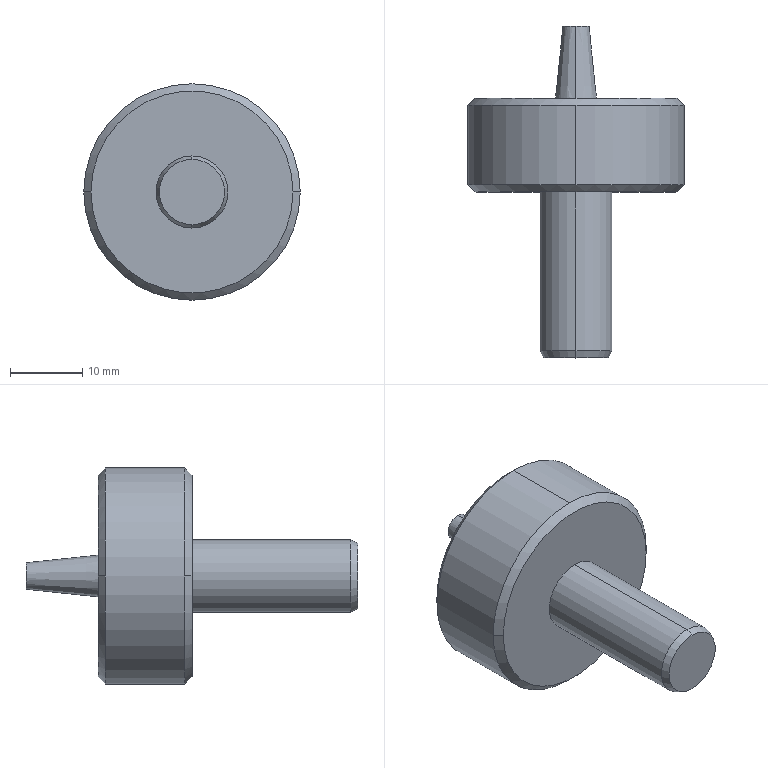Part | SolidWorks | features BaseBody 1 | 1 solid | 19 faces | box 30 x 46 x 30 mm | volume 10612 mm3 | cone 8 | cylinder 6 | plane 5 | commonest cylinder face diameters 10 x2 25 x2 30 x2
STEP:
#1=CARTESIAN_POINT('',(-418.,-55.,252.121));
#2=VERTEX_POINT('',#1);
#3=CARTESIAN_POINT('',(-418.,-55.,242.121));
#4=VERTEX_POINT('',#3);
#5=CARTESIAN_POINT('',(-418.,-55.,247.121));
#6=DIRECTION('',(0.,1.,0.));
#7=DIRECTION('',(0.,0.,-1.));
#8=AXIS2_PLACEMENT_3D('',#5,#6,#7);
#9=CIRCLE('',#8,5.);
#10=EDGE_CURVE('',#2,#4,#9,.T.);
#11=ORIENTED_EDGE('',*,*,#10,.F.);
#12=CARTESIAN_POINT('',(-418.,-77.,252.121));
#13=VERTEX_POINT('',#12);
#14=CARTESIAN_POINT('',(-418.,-78.,252.121));
#15=DIRECTION('',(0.,-1.,0.));
#16=VECTOR('',#15,1000.);
#17=LINE('',#14,#16);
#18=EDGE_CURVE('',#2,#13,#17,.T.);
#19=ORIENTED_EDGE('',*,*,#18,.T.);
#20=CARTESIAN_POINT('',(-418.,-77.,242.121));
#21=VERTEX_POINT('',#20);
#22=CARTESIAN_POINT('',(-418.,-77.,247.121));
#23=DIRECTION('',(0.,1.,0.));
#24=DIRECTION('',(0.,0.,-1.));
#25=AXIS2_PLACEMENT_3D('',#22,#23,#24);
#26=CIRCLE('',#25,5.);
#27=EDGE_CURVE('',#13,#21,#26,.T.);
#28=ORIENTED_EDGE('',*,*,#27,.T.);
#29=CARTESIAN_POINT('',(-418.,-78.,242.121));
#30=DIRECTION('',(0.,-1.,0.));
#31=VECTOR('',#30,1000.);
#32=LINE('',#29,#31);
#33=EDGE_CURVE('',#4,#21,#32,.T.);
#34=ORIENTED_EDGE('',*,*,#33,.F.);
#35=EDGE_LOOP('',(#11,#19,#28,#34));
#36=FACE_OUTER_BOUND('',#35,.T.);
#37=CARTESIAN_POINT('',(-418.,-78.,247.121));
#38=DIRECTION('',(0.,-1.,0.));
#39=DIRECTION('',(0.,0.,-1.));
#40=AXIS2_PLACEMENT_3D('',#37,#38,#39);
#41=CYLINDRICAL_SURFACE('',#40,5.);
#42=ADVANCED_FACE('',(#36),#41,.T.);
#43=CARTESIAN_POINT('',(-404.,-55.,247.121));
#44=VERTEX_POINT('',#43);
#45=CARTESIAN_POINT('',(-432.,-55.,247.121));
#46=VERTEX_POINT('',#45);
#47=CARTESIAN_POINT('',(-418.,-55.,247.121));
#48=DIRECTION('',(0.,-1.,0.));
#49=DIRECTION('',(-1.,0.,0.));
#50=AXIS2_PLACEMENT_3D('',#47,#48,#49);
#51=CIRCLE('',#50,14.);
#52=EDGE_CURVE('',#44,#46,#51,.T.);
#53=ORIENTED_EDGE('',*,*,#52,.F.);
#54=CARTESIAN_POINT('',(-403.,-54.,247.121));
#55=VERTEX_POINT('',#54);
#56=CARTESIAN_POINT('',(-403.,-54.,247.121));
#57=DIRECTION('',(0.7071,0.7071,0.));
#58=VECTOR('',#57,1000.);
#59=LINE('',#56,#58);
#60=EDGE_CURVE('',#44,#55,#59,.T.);
#61=ORIENTED_EDGE('',*,*,#60,.T.);
#62=CARTESIAN_POINT('',(-418.,-54.,262.121));
#63=VERTEX_POINT('',#62);
#64=CARTESIAN_POINT('',(-418.,-54.,247.121));
#65=DIRECTION('',(0.,-1.,0.));
#66=DIRECTION('',(0.114,0.,-0.9935));
#67=AXIS2_PLACEMENT_3D('',#64,#65,#66);
#68=CIRCLE('',#67,15.);
#69=EDGE_CURVE('',#55,#63,#68,.T.);
#70=ORIENTED_EDGE('',*,*,#69,.T.);
#71=CARTESIAN_POINT('',(-433.,-54.,247.121));
#72=VERTEX_POINT('',#71);
#73=CARTESIAN_POINT('',(-418.,-54.,247.121));
#74=DIRECTION('',(0.,-1.,0.));
#75=DIRECTION('',(0.114,0.,-0.9935));
#76=AXIS2_PLACEMENT_3D('',#73,#74,#75);
#77=CIRCLE('',#76,15.);
#78=EDGE_CURVE('',#63,#72,#77,.T.);
#79=ORIENTED_EDGE('',*,*,#78,.T.);
#80=CARTESIAN_POINT('',(-433.,-54.,247.121));
#81=DIRECTION('',(-0.7071,0.7071,0.));
#82=VECTOR('',#81,1000.);
#83=LINE('',#80,#82);
#84=EDGE_CURVE('',#46,#72,#83,.T.);
#85=ORIENTED_EDGE('',*,*,#84,.F.);
#86=EDGE_LOOP('',(#53,#61,#70,#79,#85));
#87=FACE_OUTER_BOUND('',#86,.T.);
#88=CARTESIAN_POINT('',(-418.,-54.,247.121));
#89=DIRECTION('',(0.,1.,0.));
#90=DIRECTION('',(-1.,0.,0.));
#91=AXIS2_PLACEMENT_3D('',#88,#89,#90);
#92=CONICAL_SURFACE('',#91,15.,0.7854);
#93=ADVANCED_FACE('',(#87),#92,.T.);
#94=CARTESIAN_POINT('',(-418.,-78.,251.655));
#95=VERTEX_POINT('',#94);
#96=CARTESIAN_POINT('',(-418.,-78.,242.587));
#97=VERTEX_POINT('',#96);
#98=CARTESIAN_POINT('',(-418.,-78.,247.121));
#99=DIRECTION('',(0.,1.,0.));
#100=DIRECTION('',(0.,0.,1.));
#101=AXIS2_PLACEMENT_3D('',#98,#99,#100);
#102=CIRCLE('',#101,4.534);
#103=EDGE_CURVE('',#95,#97,#102,.T.);
#104=ORIENTED_EDGE('',*,*,#103,.T.);
#105=CARTESIAN_POINT('',(-418.,-77.,242.121));
#106=DIRECTION('',(0.,0.9063,-0.4226));
#107=VECTOR('',#106,1000.);
#108=LINE('',#105,#107);
#109=EDGE_CURVE('',#97,#21,#108,.T.);
#110=ORIENTED_EDGE('',*,*,#109,.T.);
#111=ORIENTED_EDGE('',*,*,#27,.F.);
#112=CARTESIAN_POINT('',(-418.,-77.,252.121));
#113=DIRECTION('',(0.,0.9063,0.4226));
#114=VECTOR('',#113,1000.);
#115=LINE('',#112,#114);
#116=EDGE_CURVE('',#95,#13,#115,.T.);
#117=ORIENTED_EDGE('',*,*,#116,.F.);
#118=EDGE_LOOP('',(#104,#110,#111,#117));
#119=FACE_OUTER_BOUND('',#118,.T.);
#120=CARTESIAN_POINT('',(-418.,-77.,247.121));
#121=DIRECTION('',(0.,1.,0.));
#122=DIRECTION('',(0.,0.,1.));
#123=AXIS2_PLACEMENT_3D('',#120,#121,#122);
#124=CONICAL_SURFACE('',#123,5.,0.4363);
#125=ADVANCED_FACE('',(#119),#124,.T.);
#126=CARTESIAN_POINT('',(-403.,-43.,247.121));
#127=VERTEX_POINT('',#126);
#128=CARTESIAN_POINT('',(-418.,-43.,262.121));
#129=VERTEX_POINT('',#128);
#130=CARTESIAN_POINT('',(-418.,-43.,247.121));
#131=DIRECTION('',(0.,-1.,0.));
#132=DIRECTION('',(0.,0.,-1.));
#133=AXIS2_PLACEMENT_3D('',#130,#131,#132);
#134=CIRCLE('',#133,15.);
#135=EDGE_CURVE('',#127,#129,#134,.T.);
#136=ORIENTED_EDGE('',*,*,#135,.T.);
#137=CARTESIAN_POINT('',(-418.,-78.,262.121));
#138=DIRECTION('',(0.,-1.,0.));
#139=VECTOR('',#138,1000.);
#140=LINE('',#137,#139);
#141=EDGE_CURVE('',#129,#63,#140,.T.);
#142=ORIENTED_EDGE('',*,*,#141,.T.);
#143=ORIENTED_EDGE('',*,*,#69,.F.);
#144=CARTESIAN_POINT('',(-418.,-54.,232.121));
#145=VERTEX_POINT('',#144);
#146=CARTESIAN_POINT('',(-418.,-54.,247.121));
#147=DIRECTION('',(0.,-1.,0.));
#148=DIRECTION('',(0.114,0.,-0.9935));
#149=AXIS2_PLACEMENT_3D('',#146,#147,#148);
#150=CIRCLE('',#149,15.);
#151=EDGE_CURVE('',#145,#55,#150,.T.);
#152=ORIENTED_EDGE('',*,*,#151,.F.);
#153=CARTESIAN_POINT('',(-418.,-43.,232.121));
#154=VERTEX_POINT('',#153);
#155=CARTESIAN_POINT('',(-418.,-78.,232.121));
#156=DIRECTION('',(0.,-1.,0.));
#157=VECTOR('',#156,1000.);
#158=LINE('',#155,#157);
#159=EDGE_CURVE('',#154,#145,#158,.T.);
#160=ORIENTED_EDGE('',*,*,#159,.F.);
#161=CARTESIAN_POINT('',(-418.,-43.,247.121));
#162=DIRECTION('',(0.,-1.,0.));
#163=DIRECTION('',(0.,0.,-1.));
#164=AXIS2_PLACEMENT_3D('',#161,#162,#163);
#165=CIRCLE('',#164,15.);
#166=EDGE_CURVE('',#154,#127,#165,.T.);
#167=ORIENTED_EDGE('',*,*,#166,.T.);
#168=EDGE_LOOP('',(#136,#142,#143,#152,#160,#167));
#169=FACE_OUTER_BOUND('',#168,.T.);
#170=CARTESIAN_POINT('',(-418.,-78.,247.121));
#171=DIRECTION('',(0.,-1.,0.));
#172=DIRECTION('',(0.,0.,-1.));
#173=AXIS2_PLACEMENT_3D('',#170,#171,#172);
#174=CYLINDRICAL_SURFACE('',#173,15.);
#175=ADVANCED_FACE('',(#169),#174,.T.);
#176=CARTESIAN_POINT('',(-404.,-42.,247.121));
#177=VERTEX_POINT('',#176);
#178=CARTESIAN_POINT('',(-432.,-42.,247.121));
#179=VERTEX_POINT('',#178);
#180=CARTESIAN_POINT('',(-418.,-42.,247.121));
#181=DIRECTION('',(0.,-1.,0.));
#182=DIRECTION('',(1.,0.,0.));
#183=AXIS2_PLACEMENT_3D('',#180,#181,#182);
#184=CIRCLE('',#183,14.);
#185=EDGE_CURVE('',#177,#179,#184,.T.);
#186=ORIENTED_EDGE('',*,*,#185,.T.);
#187=CARTESIAN_POINT('',(-433.,-43.,247.121));
#188=VERTEX_POINT('',#187);
#189=CARTESIAN_POINT('',(-433.,-43.,247.121));
#190=DIRECTION('',(-0.7071,-0.7071,0.));
#191=VECTOR('',#190,1000.);
#192=LINE('',#189,#191);
#193=EDGE_CURVE('',#179,#188,#192,.T.);
#194=ORIENTED_EDGE('',*,*,#193,.T.);
#195=CARTESIAN_POINT('',(-418.,-43.,247.121));
#196=DIRECTION('',(0.,-1.,0.));
#197=DIRECTION('',(0.,0.,-1.));
#198=AXIS2_PLACEMENT_3D('',#195,#196,#197);
#199=CIRCLE('',#198,15.);
#200=EDGE_CURVE('',#129,#188,#199,.T.);
#201=ORIENTED_EDGE('',*,*,#200,.F.);
#202=ORIENTED_EDGE('',*,*,#135,.F.);
#203=CARTESIAN_POINT('',(-403.,-43.,247.121));
#204=DIRECTION('',(0.7071,-0.7071,0.));
#205=VECTOR('',#204,1000.);
#206=LINE('',#203,#205);
#207=EDGE_CURVE('',#177,#127,#206,.T.);
#208=ORIENTED_EDGE('',*,*,#207,.F.);
#209=EDGE_LOOP('',(#186,#194,#201,#202,#208));
#210=FACE_OUTER_BOUND('',#209,.T.);
#211=CARTESIAN_POINT('',(-418.,-43.,247.121));
#212=DIRECTION('',(0.,-1.,0.));
#213=DIRECTION('',(1.,0.,0.));
#214=AXIS2_PLACEMENT_3D('',#211,#212,#213);
#215=CONICAL_SURFACE('',#214,15.,0.7854);
#216=ADVANCED_FACE('',(#210),#215,.T.);
#217=CARTESIAN_POINT('',(-418.,-43.,234.621));
#218=VERTEX_POINT('',#217);
#219=CARTESIAN_POINT('',(-418.,-43.,259.621));
#220=VERTEX_POINT('',#219);
#221=CARTESIAN_POINT('',(-418.,-43.,247.121));
#222=DIRECTION('',(0.,1.,0.));
#223=DIRECTION('',(0.,0.,1.));
#224=AXIS2_PLACEMENT_3D('',#221,#222,#223);
#225=CIRCLE('',#224,12.5);
#226=EDGE_CURVE('',#218,#220,#225,.T.);
#227=ORIENTED_EDGE('',*,*,#226,.F.);
#228=CARTESIAN_POINT('',(-418.,-42.,234.621));
#229=VERTEX_POINT('',#228);
#230=CARTESIAN_POINT('',(-418.,-43.,234.621));
#231=DIRECTION('',(0.,1.,0.));
#232=VECTOR('',#231,1000.);
#233=LINE('',#230,#232);
#234=EDGE_CURVE('',#218,#229,#233,.T.);
#235=ORIENTED_EDGE('',*,*,#234,.T.);
#236=CARTESIAN_POINT('',(-418.,-42.,259.621));
#237=VERTEX_POINT('',#236);
#238=CARTESIAN_POINT('',(-418.,-42.,247.121));
#239=DIRECTION('',(0.,-1.,0.));
#240=DIRECTION('',(0.,0.,1.));
#241=AXIS2_PLACEMENT_3D('',#238,#239,#240);
#242=CIRCLE('',#241,12.5);
#243=EDGE_CURVE('',#237,#229,#242,.T.);
#244=ORIENTED_EDGE('',*,*,#243,.F.);
#245=CARTESIAN_POINT('',(-418.,-43.,259.621));
#246=DIRECTION('',(0.,1.,0.));
#247=VECTOR('',#246,1000.);
#248=LINE('',#245,#247);
#249=EDGE_CURVE('',#220,#237,#248,.T.);
#250=ORIENTED_EDGE('',*,*,#249,.F.);
#251=EDGE_LOOP('',(#227,#235,#244,#250));
#252=FACE_OUTER_BOUND('',#251,.T.);
#253=CARTESIAN_POINT('',(-418.,-43.,247.121));
#254=DIRECTION('',(0.,1.,0.));
#255=DIRECTION('',(0.,0.,1.));
#256=AXIS2_PLACEMENT_3D('',#253,#254,#255);
#257=CYLINDRICAL_SURFACE('',#256,12.5);
#258=ADVANCED_FACE('',(#252),#257,.F.);
#259=CARTESIAN_POINT('',(-418.,-32.,245.277));
#260=VERTEX_POINT('',#259);
#261=CARTESIAN_POINT('',(-418.,-32.,248.965));
#262=VERTEX_POINT('',#261);
#263=CARTESIAN_POINT('',(-418.,-32.,247.121));
#264=DIRECTION('',(0.,-1.,0.));
#265=DIRECTION('',(0.,0.,-1.));
#266=AXIS2_PLACEMENT_3D('',#263,#264,#265);
#267=CIRCLE('',#266,1.844);
#268=EDGE_CURVE('',#260,#262,#267,.T.);
#269=ORIENTED_EDGE('',*,*,#268,.T.);
#270=CARTESIAN_POINT('',(-418.,-43.,250.121));
#271=VERTEX_POINT('',#270);
#272=CARTESIAN_POINT('',(-418.,-43.,250.121));
#273=DIRECTION('',(0.,-0.9945,0.1045));
#274=VECTOR('',#273,1000.);
#275=LINE('',#272,#274);
#276=EDGE_CURVE('',#262,#271,#275,.T.);
#277=ORIENTED_EDGE('',*,*,#276,.T.);
#278=CARTESIAN_POINT('',(-418.,-43.,244.121));
#279=VERTEX_POINT('',#278);
#280=CARTESIAN_POINT('',(-418.,-43.,247.121));
#281=DIRECTION('',(0.,-1.,0.));
#282=DIRECTION('',(0.,0.,-1.));
#283=AXIS2_PLACEMENT_3D('',#280,#281,#282);
#284=CIRCLE('',#283,3.);
#285=EDGE_CURVE('',#279,#271,#284,.T.);
#286=ORIENTED_EDGE('',*,*,#285,.F.);
#287=CARTESIAN_POINT('',(-418.,-43.,244.121));
#288=DIRECTION('',(0.,-0.9945,-0.1045));
#289=VECTOR('',#288,1000.);
#290=LINE('',#287,#289);
#291=EDGE_CURVE('',#260,#279,#290,.T.);
#292=ORIENTED_EDGE('',*,*,#291,.F.);
#293=EDGE_LOOP('',(#269,#277,#286,#292));
#294=FACE_OUTER_BOUND('',#293,.T.);
#295=CARTESIAN_POINT('',(-418.,-43.,247.121));
#296=DIRECTION('',(0.,-1.,0.));
#297=DIRECTION('',(0.,0.,-1.));
#298=AXIS2_PLACEMENT_3D('',#295,#296,#297);
#299=CONICAL_SURFACE('',#298,3.,0.1047);
#300=ADVANCED_FACE('',(#294),#299,.T.);
#301=CARTESIAN_POINT('',(-418.,-55.,247.121));
#302=DIRECTION('',(0.,1.,0.));
#303=DIRECTION('',(0.,0.,-1.));
#304=AXIS2_PLACEMENT_3D('',#301,#302,#303);
#305=CIRCLE('',#304,5.);
#306=EDGE_CURVE('',#4,#2,#305,.T.);
#307=ORIENTED_EDGE('',*,*,#306,.T.);
#308=ORIENTED_EDGE('',*,*,#10,.T.);
#309=EDGE_LOOP('',(#307,#308));
#310=FACE_BOUND('',#309,.T.);
#311=CARTESIAN_POINT('',(-418.,-55.,247.121));
#312=DIRECTION('',(0.,-1.,0.));
#313=DIRECTION('',(-1.,0.,0.));
#314=AXIS2_PLACEMENT_3D('',#311,#312,#313);
#315=CIRCLE('',#314,14.);
#316=EDGE_CURVE('',#46,#44,#315,.T.);
#317=ORIENTED_EDGE('',*,*,#316,.T.);
#318=ORIENTED_EDGE('',*,*,#52,.T.);
#319=EDGE_LOOP('',(#317,#318));
#320=FACE_OUTER_BOUND('',#319,.T.);
#321=CARTESIAN_POINT('',(-419.71,-55.,262.023));
#322=DIRECTION('',(0.,-1.,0.));
#323=DIRECTION('',(0.,0.,-1.));
#324=AXIS2_PLACEMENT_3D('',#321,#322,#323);
#325=PLANE('',#324);
#326=ADVANCED_FACE('',(#310,#320),#325,.T.);
#327=ORIENTED_EDGE('',*,*,#18,.F.);
#328=ORIENTED_EDGE('',*,*,#306,.F.);
#329=ORIENTED_EDGE('',*,*,#33,.T.);
#330=CARTESIAN_POINT('',(-418.,-77.,247.121));
#331=DIRECTION('',(0.,1.,0.));
#332=DIRECTION('',(0.,0.,-1.));
#333=AXIS2_PLACEMENT_3D('',#330,#331,#332);
#334=CIRCLE('',#333,5.);
#335=EDGE_CURVE('',#21,#13,#334,.T.);
#336=ORIENTED_EDGE('',*,*,#335,.T.);
#337=EDGE_LOOP('',(#327,#328,#329,#336));
#338=FACE_OUTER_BOUND('',#337,.T.);
#339=CARTESIAN_POINT('',(-418.,-78.,247.121));
#340=DIRECTION('',(0.,-1.,0.));
#341=DIRECTION('',(0.,0.,-1.));
#342=AXIS2_PLACEMENT_3D('',#339,#340,#341);
#343=CYLINDRICAL_SURFACE('',#342,5.);
#344=ADVANCED_FACE('',(#338),#343,.T.);
#345=ORIENTED_EDGE('',*,*,#60,.F.);
#346=ORIENTED_EDGE('',*,*,#316,.F.);
#347=ORIENTED_EDGE('',*,*,#84,.T.);
#348=CARTESIAN_POINT('',(-418.,-54.,247.121));
#349=DIRECTION('',(0.,-1.,0.));
#350=DIRECTION('',(0.114,0.,-0.9935));
#351=AXIS2_PLACEMENT_3D('',#348,#349,#350);
#352=CIRCLE('',#351,15.);
#353=EDGE_CURVE('',#72,#145,#352,.T.);
#354=ORIENTED_EDGE('',*,*,#353,.T.);
#355=ORIENTED_EDGE('',*,*,#151,.T.);
#356=EDGE_LOOP('',(#345,#346,#347,#354,#355));
#357=FACE_OUTER_BOUND('',#356,.T.);
#358=CARTESIAN_POINT('',(-418.,-54.,247.121));
#359=DIRECTION('',(0.,1.,0.));
#360=DIRECTION('',(-1.,0.,0.));
#361=AXIS2_PLACEMENT_3D('',#358,#359,#360);
#362=CONICAL_SURFACE('',#361,15.,0.7854);
#363=ADVANCED_FACE('',(#357),#362,.T.);
#364=ORIENTED_EDGE('',*,*,#109,.F.);
#365=CARTESIAN_POINT('',(-418.,-78.,247.121));
#366=DIRECTION('',(0.,1.,0.));
#367=DIRECTION('',(0.,0.,1.));
#368=AXIS2_PLACEMENT_3D('',#365,#366,#367);
#369=CIRCLE('',#368,4.534);
#370=EDGE_CURVE('',#97,#95,#369,.T.);
#371=ORIENTED_EDGE('',*,*,#370,.T.);
#372=ORIENTED_EDGE('',*,*,#116,.T.);
#373=ORIENTED_EDGE('',*,*,#335,.F.);
#374=EDGE_LOOP('',(#364,#371,#372,#373));
#375=FACE_OUTER_BOUND('',#374,.T.);
#376=CARTESIAN_POINT('',(-418.,-77.,247.121));
#377=DIRECTION('',(0.,1.,0.));
#378=DIRECTION('',(0.,0.,1.));
#379=AXIS2_PLACEMENT_3D('',#376,#377,#378);
#380=CONICAL_SURFACE('',#379,5.,0.4363);
#381=ADVANCED_FACE('',(#375),#380,.T.);
#382=ORIENTED_EDGE('',*,*,#141,.F.);
#383=ORIENTED_EDGE('',*,*,#200,.T.);
#384=CARTESIAN_POINT('',(-418.,-43.,247.121));
#385=DIRECTION('',(0.,-1.,0.));
#386=DIRECTION('',(0.,0.,-1.));
#387=AXIS2_PLACEMENT_3D('',#384,#385,#386);
#388=CIRCLE('',#387,15.);
#389=EDGE_CURVE('',#188,#154,#388,.T.);
#390=ORIENTED_EDGE('',*,*,#389,.T.);
#391=ORIENTED_EDGE('',*,*,#159,.T.);
#392=ORIENTED_EDGE('',*,*,#353,.F.);
#393=ORIENTED_EDGE('',*,*,#78,.F.);
#394=EDGE_LOOP('',(#382,#383,#390,#391,#392,#393));
#395=FACE_OUTER_BOUND('',#394,.T.);
#396=CARTESIAN_POINT('',(-418.,-78.,247.121));
#397=DIRECTION('',(0.,-1.,0.));
#398=DIRECTION('',(0.,0.,-1.));
#399=AXIS2_PLACEMENT_3D('',#396,#397,#398);
#400=CYLINDRICAL_SURFACE('',#399,15.);
#401=ADVANCED_FACE('',(#395),#400,.T.);
#402=ORIENTED_EDGE('',*,*,#103,.F.);
#403=ORIENTED_EDGE('',*,*,#370,.F.);
#404=EDGE_LOOP('',(#402,#403));
#405=FACE_OUTER_BOUND('',#404,.T.);
#406=CARTESIAN_POINT('',(-418.57,-78.,252.088));
#407=DIRECTION('',(0.,-1.,0.));
#408=DIRECTION('',(0.,0.,-1.));
#409=AXIS2_PLACEMENT_3D('',#406,#407,#408);
#410=PLANE('',#409);
#411=ADVANCED_FACE('',(#405),#410,.T.);
#412=ORIENTED_EDGE('',*,*,#193,.F.);
#413=CARTESIAN_POINT('',(-418.,-42.,247.121));
#414=DIRECTION('',(0.,-1.,0.));
#415=DIRECTION('',(1.,0.,0.));
#416=AXIS2_PLACEMENT_3D('',#413,#414,#415);
#417=CIRCLE('',#416,14.);
#418=EDGE_CURVE('',#179,#177,#417,.T.);
#419=ORIENTED_EDGE('',*,*,#418,.T.);
#420=ORIENTED_EDGE('',*,*,#207,.T.);
#421=ORIENTED_EDGE('',*,*,#166,.F.);
#422=ORIENTED_EDGE('',*,*,#389,.F.);
#423=EDGE_LOOP('',(#412,#419,#420,#421,#422));
#424=FACE_OUTER_BOUND('',#423,.T.);
#425=CARTESIAN_POINT('',(-418.,-43.,247.121));
#426=DIRECTION('',(0.,-1.,0.));
#427=DIRECTION('',(1.,0.,0.));
#428=AXIS2_PLACEMENT_3D('',#425,#426,#427);
#429=CONICAL_SURFACE('',#428,15.,0.7854);
#430=ADVANCED_FACE('',(#424),#429,.T.);
#431=ORIENTED_EDGE('',*,*,#185,.F.);
#432=ORIENTED_EDGE('',*,*,#418,.F.);
#433=EDGE_LOOP('',(#431,#432));
#434=FACE_OUTER_BOUND('',#433,.T.);
#435=ORIENTED_EDGE('',*,*,#243,.T.);
#436=CARTESIAN_POINT('',(-418.,-42.,247.121));
#437=DIRECTION('',(0.,-1.,0.));
#438=DIRECTION('',(0.,0.,1.));
#439=AXIS2_PLACEMENT_3D('',#436,#437,#438);
#440=CIRCLE('',#439,12.5);
#441=EDGE_CURVE('',#229,#237,#440,.T.);
#442=ORIENTED_EDGE('',*,*,#441,.T.);
#443=EDGE_LOOP('',(#435,#442));
#444=FACE_BOUND('',#443,.T.);
#445=CARTESIAN_POINT('',(-418.,-42.,247.121));
#446=DIRECTION('',(0.,1.,0.));
#447=DIRECTION('',(0.,0.,1.));
#448=AXIS2_PLACEMENT_3D('',#445,#446,#447);
#449=PLANE('',#448);
#450=ADVANCED_FACE('',(#434,#444),#449,.T.);
#451=ORIENTED_EDGE('',*,*,#234,.F.);
#452=CARTESIAN_POINT('',(-418.,-43.,247.121));
#453=DIRECTION('',(0.,1.,0.));
#454=DIRECTION('',(0.,0.,1.));
#455=AXIS2_PLACEMENT_3D('',#452,#453,#454);
#456=CIRCLE('',#455,12.5);
#457=EDGE_CURVE('',#220,#218,#456,.T.);
#458=ORIENTED_EDGE('',*,*,#457,.F.);
#459=ORIENTED_EDGE('',*,*,#249,.T.);
#460=ORIENTED_EDGE('',*,*,#441,.F.);
#461=EDGE_LOOP('',(#451,#458,#459,#460));
#462=FACE_OUTER_BOUND('',#461,.T.);
#463=CARTESIAN_POINT('',(-418.,-43.,247.121));
#464=DIRECTION('',(0.,1.,0.));
#465=DIRECTION('',(0.,0.,1.));
#466=AXIS2_PLACEMENT_3D('',#463,#464,#465);
#467=CYLINDRICAL_SURFACE('',#466,12.5);
#468=ADVANCED_FACE('',(#462),#467,.F.);
#469=ORIENTED_EDGE('',*,*,#285,.T.);
#470=CARTESIAN_POINT('',(-418.,-43.,247.121));
#471=DIRECTION('',(0.,-1.,0.));
#472=DIRECTION('',(0.,0.,-1.));
#473=AXIS2_PLACEMENT_3D('',#470,#471,#472);
#474=CIRCLE('',#473,3.);
#475=EDGE_CURVE('',#271,#279,#474,.T.);
#476=ORIENTED_EDGE('',*,*,#475,.T.);
#477=EDGE_LOOP('',(#469,#476));
#478=FACE_BOUND('',#477,.T.);
#479=ORIENTED_EDGE('',*,*,#457,.T.);
#480=ORIENTED_EDGE('',*,*,#226,.T.);
#481=EDGE_LOOP('',(#479,#480));
#482=FACE_OUTER_BOUND('',#481,.T.);
#483=CARTESIAN_POINT('',(-418.,-43.,247.121));
#484=DIRECTION('',(0.,1.,0.));
#485=DIRECTION('',(0.,0.,1.));
#486=AXIS2_PLACEMENT_3D('',#483,#484,#485);
#487=PLANE('',#486);
#488=ADVANCED_FACE('',(#478,#482),#487,.T.);
#489=ORIENTED_EDGE('',*,*,#276,.F.);
#490=CARTESIAN_POINT('',(-418.,-32.,247.121));
#491=DIRECTION('',(0.,-1.,0.));
#492=DIRECTION('',(0.,0.,-1.));
#493=AXIS2_PLACEMENT_3D('',#490,#491,#492);
#494=CIRCLE('',#493,1.844);
#495=EDGE_CURVE('',#262,#260,#494,.T.);
#496=ORIENTED_EDGE('',*,*,#495,.T.);
#497=ORIENTED_EDGE('',*,*,#291,.T.);
#498=ORIENTED_EDGE('',*,*,#475,.F.);
#499=EDGE_LOOP('',(#489,#496,#497,#498));
#500=FACE_OUTER_BOUND('',#499,.T.);
#501=CARTESIAN_POINT('',(-418.,-43.,247.121));
#502=DIRECTION('',(0.,-1.,0.));
#503=DIRECTION('',(0.,0.,-1.));
#504=AXIS2_PLACEMENT_3D('',#501,#502,#503);
#505=CONICAL_SURFACE('',#504,3.,0.1047);
#506=ADVANCED_FACE('',(#500),#505,.T.);
#507=ORIENTED_EDGE('',*,*,#268,.F.);
#508=ORIENTED_EDGE('',*,*,#495,.F.);
#509=EDGE_LOOP('',(#507,#508));
#510=FACE_OUTER_BOUND('',#509,.T.);
#511=CARTESIAN_POINT('',(-418.,-32.,247.121));
#512=DIRECTION('',(0.,1.,0.));
#513=DIRECTION('',(0.,0.,1.));
#514=AXIS2_PLACEMENT_3D('',#511,#512,#513);
#515=PLANE('',#514);
#516=ADVANCED_FACE('',(#510),#515,.T.);
#517=CLOSED_SHELL('',(#42,#93,#125,#175,#216,#258,#300,#326,#344,#363,#381,#401,#411,#430,#450,#468,#488,#506,#516));
#518=MANIFOLD_SOLID_BREP('',#517);
#519=CARTESIAN_POINT('',(0.,0.,0.));
#520=DIRECTION('',(0.,0.,1.));
#521=DIRECTION('',(1.,0.,0.));
#522=AXIS2_PLACEMENT_3D('',#519,#520,#521);
#523=(LENGTH_UNIT()NAMED_UNIT(*)SI_UNIT(.MILLI.,.METRE.));
#524=UNCERTAINTY_MEASURE_WITH_UNIT(LENGTH_MEASURE(0.00001),#523,'','');
#525=(NAMED_UNIT(*)PLANE_ANGLE_UNIT()SI_UNIT($,.RADIAN.));
#526=(NAMED_UNIT(*)SI_UNIT($,.STERADIAN.)SOLID_ANGLE_UNIT());
#527=(GEOMETRIC_REPRESENTATION_CONTEXT(3)GLOBAL_UNCERTAINTY_ASSIGNED_CONTEXT((#524))GLOBAL_UNIT_ASSIGNED_CONTEXT((#523,#525,#526))REPRESENTATION_CONTEXT('',''));
#528=ADVANCED_BREP_SHAPE_REPRESENTATION('',(#518,#522),#527);